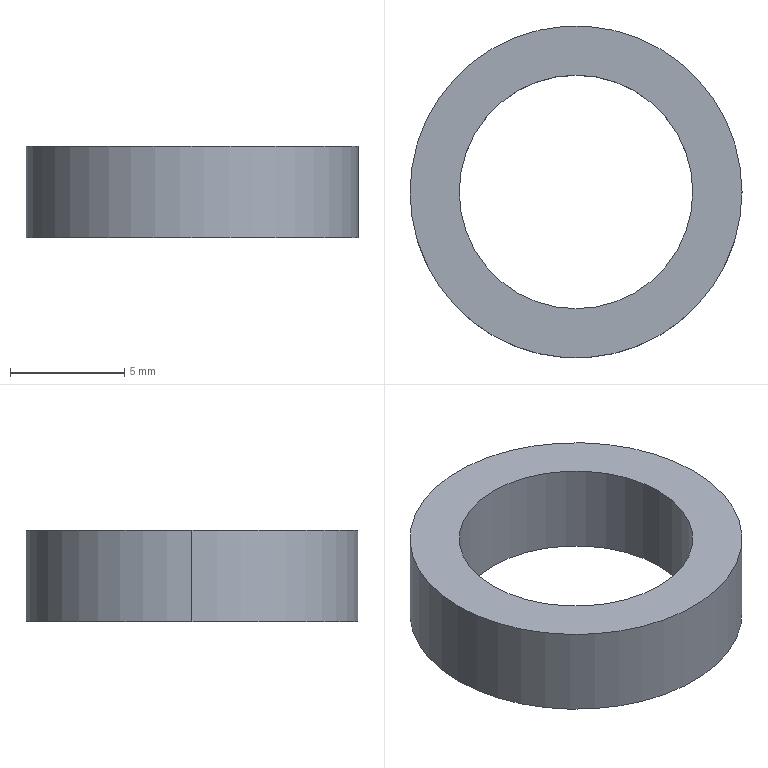Part | SolidWorks | features Revolution 1 | 1 solid | 6 faces | box 14.5 x 14.5 x 4 mm | volume 333.669 mm3 | cylinder 4 | plane 2 | commonest cylinder face diameters 10.2 x2 14.5 x2
STEP:
#1=CARTESIAN_POINT('',(-7.25,0.,2.));
#2=VERTEX_POINT('',#1);
#3=CARTESIAN_POINT('',(7.25,0.,2.));
#4=VERTEX_POINT('',#3);
#5=CARTESIAN_POINT('',(0.,0.,2.));
#6=DIRECTION('',(0.,0.,-1.));
#7=DIRECTION('',(-1.,0.,0.));
#8=AXIS2_PLACEMENT_3D('',#5,#6,#7);
#9=CIRCLE('',#8,7.25);
#10=EDGE_CURVE('',#2,#4,#9,.T.);
#11=ORIENTED_EDGE('',*,*,#10,.T.);
#12=CARTESIAN_POINT('',(7.25,0.,-2.));
#13=VERTEX_POINT('',#12);
#14=CARTESIAN_POINT('',(7.25,0.,2.));
#15=DIRECTION('',(0.,0.,-1.));
#16=VECTOR('',#15,1000.);
#17=LINE('',#14,#16);
#18=EDGE_CURVE('',#4,#13,#17,.T.);
#19=ORIENTED_EDGE('',*,*,#18,.T.);
#20=CARTESIAN_POINT('',(-7.25,0.,-2.));
#21=VERTEX_POINT('',#20);
#22=CARTESIAN_POINT('',(0.,0.,-2.));
#23=DIRECTION('',(0.,0.,-1.));
#24=DIRECTION('',(-1.,0.,0.));
#25=AXIS2_PLACEMENT_3D('',#22,#23,#24);
#26=CIRCLE('',#25,7.25);
#27=EDGE_CURVE('',#21,#13,#26,.T.);
#28=ORIENTED_EDGE('',*,*,#27,.F.);
#29=CARTESIAN_POINT('',(-7.25,0.,2.));
#30=DIRECTION('',(0.,0.,-1.));
#31=VECTOR('',#30,1000.);
#32=LINE('',#29,#31);
#33=EDGE_CURVE('',#2,#21,#32,.T.);
#34=ORIENTED_EDGE('',*,*,#33,.F.);
#35=EDGE_LOOP('',(#11,#19,#28,#34));
#36=FACE_OUTER_BOUND('',#35,.T.);
#37=CARTESIAN_POINT('',(0.,0.,2.));
#38=DIRECTION('',(0.,0.,-1.));
#39=DIRECTION('',(-1.,0.,0.));
#40=AXIS2_PLACEMENT_3D('',#37,#38,#39);
#41=CYLINDRICAL_SURFACE('',#40,7.25);
#42=ADVANCED_FACE('',(#36),#41,.T.);
#43=CARTESIAN_POINT('',(5.1,0.,2.));
#44=VERTEX_POINT('',#43);
#45=CARTESIAN_POINT('',(-5.1,0.,2.));
#46=VERTEX_POINT('',#45);
#47=CARTESIAN_POINT('',(0.,0.,2.));
#48=DIRECTION('',(0.,0.,-1.));
#49=DIRECTION('',(-1.,0.,0.));
#50=AXIS2_PLACEMENT_3D('',#47,#48,#49);
#51=CIRCLE('',#50,5.1);
#52=EDGE_CURVE('',#44,#46,#51,.T.);
#53=ORIENTED_EDGE('',*,*,#52,.F.);
#54=CARTESIAN_POINT('',(5.1,0.,-2.));
#55=VERTEX_POINT('',#54);
#56=CARTESIAN_POINT('',(5.1,0.,2.));
#57=DIRECTION('',(0.,0.,-1.));
#58=VECTOR('',#57,1000.);
#59=LINE('',#56,#58);
#60=EDGE_CURVE('',#44,#55,#59,.T.);
#61=ORIENTED_EDGE('',*,*,#60,.T.);
#62=CARTESIAN_POINT('',(-5.1,0.,-2.));
#63=VERTEX_POINT('',#62);
#64=CARTESIAN_POINT('',(0.,0.,-2.));
#65=DIRECTION('',(0.,0.,-1.));
#66=DIRECTION('',(-1.,0.,0.));
#67=AXIS2_PLACEMENT_3D('',#64,#65,#66);
#68=CIRCLE('',#67,5.1);
#69=EDGE_CURVE('',#55,#63,#68,.T.);
#70=ORIENTED_EDGE('',*,*,#69,.T.);
#71=CARTESIAN_POINT('',(-5.1,0.,2.));
#72=DIRECTION('',(0.,0.,-1.));
#73=VECTOR('',#72,1000.);
#74=LINE('',#71,#73);
#75=EDGE_CURVE('',#46,#63,#74,.T.);
#76=ORIENTED_EDGE('',*,*,#75,.F.);
#77=EDGE_LOOP('',(#53,#61,#70,#76));
#78=FACE_OUTER_BOUND('',#77,.T.);
#79=CARTESIAN_POINT('',(0.,0.,2.));
#80=DIRECTION('',(0.,0.,-1.));
#81=DIRECTION('',(-1.,0.,0.));
#82=AXIS2_PLACEMENT_3D('',#79,#80,#81);
#83=CYLINDRICAL_SURFACE('',#82,5.1);
#84=ADVANCED_FACE('',(#78),#83,.F.);
#85=ORIENTED_EDGE('',*,*,#60,.F.);
#86=CARTESIAN_POINT('',(0.,0.,2.));
#87=DIRECTION('',(0.,0.,-1.));
#88=DIRECTION('',(-1.,0.,0.));
#89=AXIS2_PLACEMENT_3D('',#86,#87,#88);
#90=CIRCLE('',#89,5.1);
#91=EDGE_CURVE('',#46,#44,#90,.T.);
#92=ORIENTED_EDGE('',*,*,#91,.F.);
#93=ORIENTED_EDGE('',*,*,#75,.T.);
#94=CARTESIAN_POINT('',(0.,0.,-2.));
#95=DIRECTION('',(0.,0.,-1.));
#96=DIRECTION('',(-1.,0.,0.));
#97=AXIS2_PLACEMENT_3D('',#94,#95,#96);
#98=CIRCLE('',#97,5.1);
#99=EDGE_CURVE('',#63,#55,#98,.T.);
#100=ORIENTED_EDGE('',*,*,#99,.T.);
#101=EDGE_LOOP('',(#85,#92,#93,#100));
#102=FACE_OUTER_BOUND('',#101,.T.);
#103=CARTESIAN_POINT('',(0.,0.,2.));
#104=DIRECTION('',(0.,0.,-1.));
#105=DIRECTION('',(-1.,0.,0.));
#106=AXIS2_PLACEMENT_3D('',#103,#104,#105);
#107=CYLINDRICAL_SURFACE('',#106,5.1);
#108=ADVANCED_FACE('',(#102),#107,.F.);
#109=ORIENTED_EDGE('',*,*,#27,.T.);
#110=CARTESIAN_POINT('',(0.,0.,-2.));
#111=DIRECTION('',(0.,0.,-1.));
#112=DIRECTION('',(-1.,0.,0.));
#113=AXIS2_PLACEMENT_3D('',#110,#111,#112);
#114=CIRCLE('',#113,7.25);
#115=EDGE_CURVE('',#13,#21,#114,.T.);
#116=ORIENTED_EDGE('',*,*,#115,.T.);
#117=EDGE_LOOP('',(#109,#116));
#118=FACE_OUTER_BOUND('',#117,.T.);
#119=ORIENTED_EDGE('',*,*,#99,.F.);
#120=ORIENTED_EDGE('',*,*,#69,.F.);
#121=EDGE_LOOP('',(#119,#120));
#122=FACE_BOUND('',#121,.T.);
#123=CARTESIAN_POINT('',(5.1,0.,-2.));
#124=DIRECTION('',(0.,0.,-1.));
#125=DIRECTION('',(-1.,0.,0.));
#126=AXIS2_PLACEMENT_3D('',#123,#124,#125);
#127=PLANE('',#126);
#128=ADVANCED_FACE('',(#118,#122),#127,.T.);
#129=ORIENTED_EDGE('',*,*,#18,.F.);
#130=CARTESIAN_POINT('',(0.,0.,2.));
#131=DIRECTION('',(0.,0.,-1.));
#132=DIRECTION('',(-1.,0.,0.));
#133=AXIS2_PLACEMENT_3D('',#130,#131,#132);
#134=CIRCLE('',#133,7.25);
#135=EDGE_CURVE('',#4,#2,#134,.T.);
#136=ORIENTED_EDGE('',*,*,#135,.T.);
#137=ORIENTED_EDGE('',*,*,#33,.T.);
#138=ORIENTED_EDGE('',*,*,#115,.F.);
#139=EDGE_LOOP('',(#129,#136,#137,#138));
#140=FACE_OUTER_BOUND('',#139,.T.);
#141=CARTESIAN_POINT('',(0.,0.,2.));
#142=DIRECTION('',(0.,0.,-1.));
#143=DIRECTION('',(-1.,0.,0.));
#144=AXIS2_PLACEMENT_3D('',#141,#142,#143);
#145=CYLINDRICAL_SURFACE('',#144,7.25);
#146=ADVANCED_FACE('',(#140),#145,.T.);
#147=ORIENTED_EDGE('',*,*,#91,.T.);
#148=ORIENTED_EDGE('',*,*,#52,.T.);
#149=EDGE_LOOP('',(#147,#148));
#150=FACE_BOUND('',#149,.T.);
#151=ORIENTED_EDGE('',*,*,#10,.F.);
#152=ORIENTED_EDGE('',*,*,#135,.F.);
#153=EDGE_LOOP('',(#151,#152));
#154=FACE_OUTER_BOUND('',#153,.T.);
#155=CARTESIAN_POINT('',(7.25,0.,2.));
#156=DIRECTION('',(0.,0.,1.));
#157=DIRECTION('',(1.,0.,0.));
#158=AXIS2_PLACEMENT_3D('',#155,#156,#157);
#159=PLANE('',#158);
#160=ADVANCED_FACE('',(#150,#154),#159,.T.);
#161=CLOSED_SHELL('',(#42,#84,#108,#128,#146,#160));
#162=MANIFOLD_SOLID_BREP('',#161);
#163=CARTESIAN_POINT('',(0.,0.,0.));
#164=DIRECTION('',(0.,0.,1.));
#165=DIRECTION('',(1.,0.,0.));
#166=AXIS2_PLACEMENT_3D('',#163,#164,#165);
#167=(LENGTH_UNIT()NAMED_UNIT(*)SI_UNIT(.MILLI.,.METRE.));
#168=UNCERTAINTY_MEASURE_WITH_UNIT(LENGTH_MEASURE(0.00001),#167,'','');
#169=(NAMED_UNIT(*)PLANE_ANGLE_UNIT()SI_UNIT($,.RADIAN.));
#170=(NAMED_UNIT(*)SI_UNIT($,.STERADIAN.)SOLID_ANGLE_UNIT());
#171=(GEOMETRIC_REPRESENTATION_CONTEXT(3)GLOBAL_UNCERTAINTY_ASSIGNED_CONTEXT((#168))GLOBAL_UNIT_ASSIGNED_CONTEXT((#167,#169,#170))REPRESENTATION_CONTEXT('',''));
#172=ADVANCED_BREP_SHAPE_REPRESENTATION('',(#162,#166),#171);